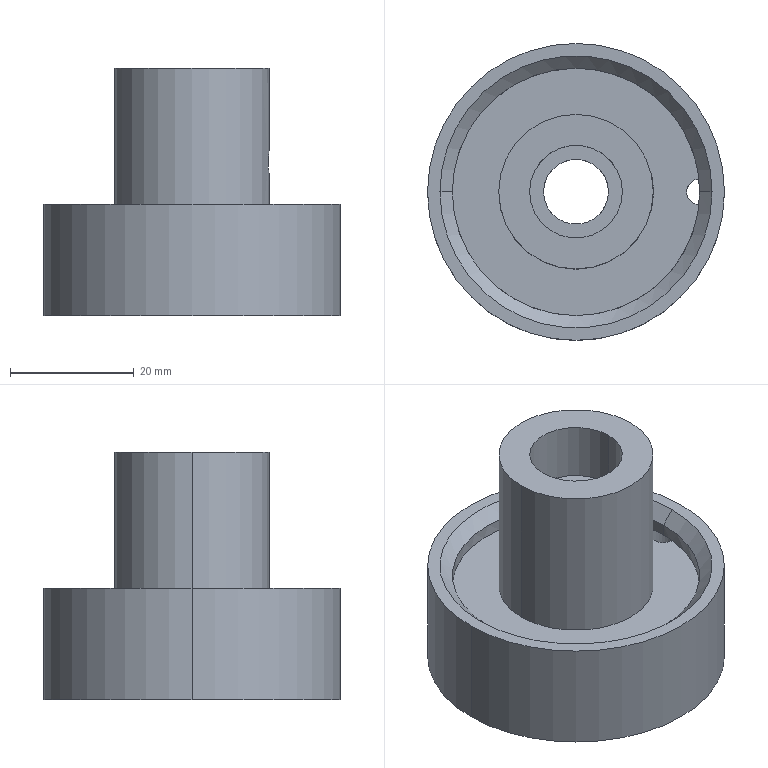Part | 1 solid | 38 faces | box 48 x 48 x 40 mm | volume 34647 mm3 | cylinder 22 | cone 8 | plane 8 | commonest cylinder face diameters 4.2 x8 10.5 x2 12 x2 12.5 x2 15 x2 25 x2
STEP:
#1=CARTESIAN_POINT('',(-6.25,0.,0.));
#2=VERTEX_POINT('',#1);
#3=CARTESIAN_POINT('',(6.25,0.,0.));
#4=VERTEX_POINT('',#3);
#5=CARTESIAN_POINT('',(0.,0.,0.));
#6=DIRECTION('',(0.,0.,1.));
#7=DIRECTION('',(1.,0.,0.));
#8=AXIS2_PLACEMENT_3D('',#5,#6,#7);
#9=CIRCLE('',#8,6.25);
#10=EDGE_CURVE('',#2,#4,#9,.T.);
#11=ORIENTED_EDGE('',*,*,#10,.F.);
#12=CARTESIAN_POINT('',(-6.25,0.,10.5));
#13=VERTEX_POINT('',#12);
#14=CARTESIAN_POINT('',(-6.25,0.,10.5));
#15=DIRECTION('',(0.,0.,1.));
#16=VECTOR('',#15,1000.);
#17=LINE('',#14,#16);
#18=EDGE_CURVE('',#2,#13,#17,.T.);
#19=ORIENTED_EDGE('',*,*,#18,.T.);
#20=CARTESIAN_POINT('',(6.25,0.,10.5));
#21=VERTEX_POINT('',#20);
#22=CARTESIAN_POINT('',(0.,0.,10.5));
#23=DIRECTION('',(0.,0.,1.));
#24=DIRECTION('',(1.,0.,0.));
#25=AXIS2_PLACEMENT_3D('',#22,#23,#24);
#26=CIRCLE('',#25,6.25);
#27=EDGE_CURVE('',#13,#21,#26,.T.);
#28=ORIENTED_EDGE('',*,*,#27,.T.);
#29=CARTESIAN_POINT('',(6.25,0.,10.5));
#30=DIRECTION('',(0.,0.,1.));
#31=VECTOR('',#30,1000.);
#32=LINE('',#29,#31);
#33=EDGE_CURVE('',#4,#21,#32,.T.);
#34=ORIENTED_EDGE('',*,*,#33,.F.);
#35=EDGE_LOOP('',(#11,#19,#28,#34));
#36=FACE_OUTER_BOUND('',#35,.T.);
#37=CARTESIAN_POINT('',(0.,0.,10.5));
#38=DIRECTION('',(0.,0.,1.));
#39=DIRECTION('',(1.,0.,0.));
#40=AXIS2_PLACEMENT_3D('',#37,#38,#39);
#41=CYLINDRICAL_SURFACE('',#40,6.25);
#42=ADVANCED_FACE('',(#36),#41,.F.);
#43=CARTESIAN_POINT('',(6.,0.,10.5));
#44=VERTEX_POINT('',#43);
#45=CARTESIAN_POINT('',(-6.,0.,10.5));
#46=VERTEX_POINT('',#45);
#47=CARTESIAN_POINT('',(0.,0.,10.5));
#48=DIRECTION('',(0.,0.,-1.));
#49=DIRECTION('',(1.,0.,0.));
#50=AXIS2_PLACEMENT_3D('',#47,#48,#49);
#51=CIRCLE('',#50,6.);
#52=EDGE_CURVE('',#44,#46,#51,.T.);
#53=ORIENTED_EDGE('',*,*,#52,.T.);
#54=CARTESIAN_POINT('',(-6.,0.,14.5));
#55=VERTEX_POINT('',#54);
#56=CARTESIAN_POINT('',(-6.,0.,10.5));
#57=DIRECTION('',(0.,0.,1.));
#58=VECTOR('',#57,1000.);
#59=LINE('',#56,#58);
#60=EDGE_CURVE('',#46,#55,#59,.T.);
#61=ORIENTED_EDGE('',*,*,#60,.T.);
#62=CARTESIAN_POINT('',(6.,0.,14.5));
#63=VERTEX_POINT('',#62);
#64=CARTESIAN_POINT('',(0.,0.,14.5));
#65=DIRECTION('',(0.,0.,1.));
#66=DIRECTION('',(1.,0.,0.));
#67=AXIS2_PLACEMENT_3D('',#64,#65,#66);
#68=CIRCLE('',#67,6.);
#69=EDGE_CURVE('',#55,#63,#68,.T.);
#70=ORIENTED_EDGE('',*,*,#69,.T.);
#71=CARTESIAN_POINT('',(6.,0.,10.5));
#72=DIRECTION('',(0.,0.,1.));
#73=VECTOR('',#72,1000.);
#74=LINE('',#71,#73);
#75=EDGE_CURVE('',#44,#63,#74,.T.);
#76=ORIENTED_EDGE('',*,*,#75,.F.);
#77=EDGE_LOOP('',(#53,#61,#70,#76));
#78=FACE_OUTER_BOUND('',#77,.T.);
#79=CARTESIAN_POINT('',(0.,0.,10.5));
#80=DIRECTION('',(0.,0.,1.));
#81=DIRECTION('',(1.,0.,0.));
#82=AXIS2_PLACEMENT_3D('',#79,#80,#81);
#83=CYLINDRICAL_SURFACE('',#82,6.);
#84=ADVANCED_FACE('',(#78),#83,.F.);
#85=CARTESIAN_POINT('',(-5.25,0.,17.5));
#86=VERTEX_POINT('',#85);
#87=CARTESIAN_POINT('',(5.25,0.,17.5));
#88=VERTEX_POINT('',#87);
#89=CARTESIAN_POINT('',(0.,0.,17.5));
#90=DIRECTION('',(0.,0.,1.));
#91=DIRECTION('',(1.,0.,0.));
#92=AXIS2_PLACEMENT_3D('',#89,#90,#91);
#93=CIRCLE('',#92,5.25);
#94=EDGE_CURVE('',#86,#88,#93,.T.);
#95=ORIENTED_EDGE('',*,*,#94,.T.);
#96=CARTESIAN_POINT('',(5.5,0.,14.5));
#97=VERTEX_POINT('',#96);
#98=CARTESIAN_POINT('',(5.5,0.,14.5));
#99=DIRECTION('',(0.08305,0.,-0.9965));
#100=VECTOR('',#99,1000.);
#101=LINE('',#98,#100);
#102=EDGE_CURVE('',#88,#97,#101,.T.);
#103=ORIENTED_EDGE('',*,*,#102,.T.);
#104=CARTESIAN_POINT('',(-5.5,0.,14.5));
#105=VERTEX_POINT('',#104);
#106=CARTESIAN_POINT('',(0.,0.,14.5));
#107=DIRECTION('',(0.,0.,1.));
#108=DIRECTION('',(1.,0.,0.));
#109=AXIS2_PLACEMENT_3D('',#106,#107,#108);
#110=CIRCLE('',#109,5.5);
#111=EDGE_CURVE('',#105,#97,#110,.T.);
#112=ORIENTED_EDGE('',*,*,#111,.F.);
#113=CARTESIAN_POINT('',(-5.5,0.,14.5));
#114=DIRECTION('',(-0.08305,0.,-0.9965));
#115=VECTOR('',#114,1000.);
#116=LINE('',#113,#115);
#117=EDGE_CURVE('',#86,#105,#116,.T.);
#118=ORIENTED_EDGE('',*,*,#117,.F.);
#119=EDGE_LOOP('',(#95,#103,#112,#118));
#120=FACE_OUTER_BOUND('',#119,.T.);
#121=CARTESIAN_POINT('',(0.,0.,14.5));
#122=DIRECTION('',(0.,0.,-1.));
#123=DIRECTION('',(-1.,0.,0.));
#124=AXIS2_PLACEMENT_3D('',#121,#122,#123);
#125=CONICAL_SURFACE('',#124,5.5,0.08314);
#126=ADVANCED_FACE('',(#120),#125,.F.);
#127=CARTESIAN_POINT('',(5.25,0.,22.7));
#128=VERTEX_POINT('',#127);
#129=CARTESIAN_POINT('',(5.25,0.,26.9));
#130=VERTEX_POINT('',#129);
#131=CARTESIAN_POINT('',(5.25,0.,22.7));
#132=CARTESIAN_POINT('',(5.25,-0.1403,22.7));
#133=CARTESIAN_POINT('',(5.244,-0.2781,22.714));
#134=CARTESIAN_POINT('',(5.223,-0.5485,22.768));
#135=CARTESIAN_POINT('',(5.207,-0.6827,22.809));
#136=CARTESIAN_POINT('',(5.167,-0.9365,22.915));
#137=CARTESIAN_POINT('',(5.144,-1.057,22.98));
#138=CARTESIAN_POINT('',(5.092,-1.284,23.133));
#139=CARTESIAN_POINT('',(5.064,-1.39,23.22));
#140=CARTESIAN_POINT('',(4.979,-1.677,23.508));
#141=CARTESIAN_POINT('',(4.921,-1.833,23.739));
#142=CARTESIAN_POINT('',(4.858,-1.991,24.117));
#143=CARTESIAN_POINT('',(4.841,-2.032,24.251));
#144=CARTESIAN_POINT('',(4.818,-2.086,24.523));
#145=CARTESIAN_POINT('',(4.812,-2.1,24.66));
#146=CARTESIAN_POINT('',(4.812,-2.1,24.937));
#147=CARTESIAN_POINT('',(4.818,-2.086,25.078));
#148=CARTESIAN_POINT('',(4.841,-2.032,25.349));
#149=CARTESIAN_POINT('',(4.858,-1.991,25.481));
#150=CARTESIAN_POINT('',(4.9,-1.885,25.736));
#151=CARTESIAN_POINT('',(4.925,-1.82,25.857));
#152=CARTESIAN_POINT('',(4.979,-1.668,26.083));
#153=CARTESIAN_POINT('',(5.007,-1.581,26.189));
#154=CARTESIAN_POINT('',(5.064,-1.388,26.382));
#155=CARTESIAN_POINT('',(5.092,-1.284,26.468));
#156=CARTESIAN_POINT('',(5.144,-1.057,26.62));
#157=CARTESIAN_POINT('',(5.168,-0.9343,26.686));
#158=CARTESIAN_POINT('',(5.227,-0.5556,26.844));
#159=CARTESIAN_POINT('',(5.25,-0.2764,26.9));
#160=CARTESIAN_POINT('',(5.25,0.,26.9));
#161=B_SPLINE_CURVE_WITH_KNOTS('',3,(#131,#132,#133,#134,#135,#136,#137,#138,#139,#140,#141,#142,#143,#144,#145,#146,#147,#148,#149,#150,#151,#152,#153,#154,#155,#156,#157,#158,#159,#160),.UNSPECIFIED.,.F.,.F.,(4,2,2,2,2,2,2,2,2,2,2,2,2,2,4),(0.,0.0004147,0.0008295,0.001244,0.001659,0.002488,0.002903,0.003318,0.003733,0.004147,0.004562,0.004977,0.005392,0.005806,0.006636),.UNSPECIFIED.);
#162=EDGE_CURVE('',#128,#130,#161,.T.);
#163=ORIENTED_EDGE('',*,*,#162,.T.);
#164=CARTESIAN_POINT('',(12.5,0.,26.9));
#165=VERTEX_POINT('',#164);
#166=CARTESIAN_POINT('',(20.,0.,26.9));
#167=DIRECTION('',(1.,0.,0.));
#168=VECTOR('',#167,1000.);
#169=LINE('',#166,#168);
#170=EDGE_CURVE('',#130,#165,#169,.T.);
#171=ORIENTED_EDGE('',*,*,#170,.T.);
#172=CARTESIAN_POINT('',(12.5,0.,22.7));
#173=VERTEX_POINT('',#172);
#174=CARTESIAN_POINT('',(12.5,0.,26.9));
#175=CARTESIAN_POINT('',(12.5,-0.2743,26.9));
#176=CARTESIAN_POINT('',(12.49,-0.5511,26.845));
#177=CARTESIAN_POINT('',(12.466,-0.9302,26.688));
#178=CARTESIAN_POINT('',(12.456,-1.053,26.622));
#179=CARTESIAN_POINT('',(12.435,-1.282,26.469));
#180=CARTESIAN_POINT('',(12.423,-1.387,26.383));
#181=CARTESIAN_POINT('',(12.4,-1.581,26.189));
#182=CARTESIAN_POINT('',(12.388,-1.669,26.081));
#183=CARTESIAN_POINT('',(12.367,-1.822,25.854));
#184=CARTESIAN_POINT('',(12.357,-1.886,25.733));
#185=CARTESIAN_POINT('',(12.34,-1.992,25.479));
#186=CARTESIAN_POINT('',(12.334,-2.032,25.346));
#187=CARTESIAN_POINT('',(12.325,-2.086,25.077));
#188=CARTESIAN_POINT('',(12.322,-2.1,24.94));
#189=CARTESIAN_POINT('',(12.322,-2.1,24.663));
#190=CARTESIAN_POINT('',(12.325,-2.087,24.526));
#191=CARTESIAN_POINT('',(12.334,-2.033,24.257));
#192=CARTESIAN_POINT('',(12.34,-1.993,24.123));
#193=CARTESIAN_POINT('',(12.357,-1.888,23.869));
#194=CARTESIAN_POINT('',(12.367,-1.823,23.749));
#195=CARTESIAN_POINT('',(12.388,-1.671,23.52));
#196=CARTESIAN_POINT('',(12.4,-1.582,23.413));
#197=CARTESIAN_POINT('',(12.434,-1.293,23.123));
#198=CARTESIAN_POINT('',(12.458,-1.059,22.966));
#199=CARTESIAN_POINT('',(12.482,-0.6803,22.809));
#200=CARTESIAN_POINT('',(12.489,-0.5475,22.768));
#201=CARTESIAN_POINT('',(12.498,-0.2763,22.714));
#202=CARTESIAN_POINT('',(12.5,-0.139,22.7));
#203=CARTESIAN_POINT('',(12.5,0.,22.7));
#204=B_SPLINE_CURVE_WITH_KNOTS('',3,(#174,#175,#176,#177,#178,#179,#180,#181,#182,#183,#184,#185,#186,#187,#188,#189,#190,#191,#192,#193,#194,#195,#196,#197,#198,#199,#200,#201,#202,#203),.UNSPECIFIED.,.F.,.F.,(4,2,2,2,2,2,2,2,2,2,2,2,2,2,4),(0.006577,0.007399,0.00781,0.008221,0.008632,0.009043,0.009454,0.009865,0.01028,0.01069,0.0111,0.01151,0.01233,0.01274,0.01315),.UNSPECIFIED.);
#205=EDGE_CURVE('',#165,#173,#204,.T.);
#206=ORIENTED_EDGE('',*,*,#205,.T.);
#207=CARTESIAN_POINT('',(20.,0.,22.7));
#208=DIRECTION('',(1.,0.,0.));
#209=VECTOR('',#208,1000.);
#210=LINE('',#207,#209);
#211=EDGE_CURVE('',#128,#173,#210,.T.);
#212=ORIENTED_EDGE('',*,*,#211,.F.);
#213=EDGE_LOOP('',(#163,#171,#206,#212));
#214=FACE_OUTER_BOUND('',#213,.T.);
#215=CARTESIAN_POINT('',(20.,0.,24.8));
#216=DIRECTION('',(1.,0.,0.));
#217=DIRECTION('',(0.,0.,-1.));
#218=AXIS2_PLACEMENT_3D('',#215,#216,#217);
#219=CYLINDRICAL_SURFACE('',#218,2.1);
#220=ADVANCED_FACE('',(#214),#219,.F.);
#221=CARTESIAN_POINT('',(-7.5,0.,30.5));
#222=VERTEX_POINT('',#221);
#223=CARTESIAN_POINT('',(7.5,0.,30.5));
#224=VERTEX_POINT('',#223);
#225=CARTESIAN_POINT('',(0.,0.,30.5));
#226=DIRECTION('',(0.,0.,1.));
#227=DIRECTION('',(1.,0.,0.));
#228=AXIS2_PLACEMENT_3D('',#225,#226,#227);
#229=CIRCLE('',#228,7.5);
#230=EDGE_CURVE('',#222,#224,#229,.T.);
#231=ORIENTED_EDGE('',*,*,#230,.F.);
#232=CARTESIAN_POINT('',(-7.5,0.,40.));
#233=VERTEX_POINT('',#232);
#234=CARTESIAN_POINT('',(-7.5,0.,30.5));
#235=DIRECTION('',(0.,0.,1.));
#236=VECTOR('',#235,1000.);
#237=LINE('',#234,#236);
#238=EDGE_CURVE('',#222,#233,#237,.T.);
#239=ORIENTED_EDGE('',*,*,#238,.T.);
#240=CARTESIAN_POINT('',(7.5,0.,40.));
#241=VERTEX_POINT('',#240);
#242=CARTESIAN_POINT('',(0.,0.,40.));
#243=DIRECTION('',(0.,0.,1.));
#244=DIRECTION('',(1.,0.,0.));
#245=AXIS2_PLACEMENT_3D('',#242,#243,#244);
#246=CIRCLE('',#245,7.5);
#247=EDGE_CURVE('',#233,#241,#246,.T.);
#248=ORIENTED_EDGE('',*,*,#247,.T.);
#249=CARTESIAN_POINT('',(7.5,0.,30.5));
#250=DIRECTION('',(0.,0.,1.));
#251=VECTOR('',#250,1000.);
#252=LINE('',#249,#251);
#253=EDGE_CURVE('',#224,#241,#252,.T.);
#254=ORIENTED_EDGE('',*,*,#253,.F.);
#255=EDGE_LOOP('',(#231,#239,#248,#254));
#256=FACE_OUTER_BOUND('',#255,.T.);
#257=CARTESIAN_POINT('',(0.,0.,30.5));
#258=DIRECTION('',(0.,0.,1.));
#259=DIRECTION('',(1.,0.,0.));
#260=AXIS2_PLACEMENT_3D('',#257,#258,#259);
#261=CYLINDRICAL_SURFACE('',#260,7.5);
#262=ADVANCED_FACE('',(#256),#261,.F.);
#263=CARTESIAN_POINT('',(-20.,0.,16.));
#264=VERTEX_POINT('',#263);
#265=CARTESIAN_POINT('',(20.,0.,16.));
#266=VERTEX_POINT('',#265);
#267=CARTESIAN_POINT('',(0.,0.,16.));
#268=DIRECTION('',(0.,0.,1.));
#269=DIRECTION('',(1.,0.,0.));
#270=AXIS2_PLACEMENT_3D('',#267,#268,#269);
#271=CIRCLE('',#270,20.);
#272=EDGE_CURVE('',#264,#266,#271,.T.);
#273=ORIENTED_EDGE('',*,*,#272,.F.);
#274=CARTESIAN_POINT('',(-22.,0.,18.));
#275=VERTEX_POINT('',#274);
#276=CARTESIAN_POINT('',(-20.,0.,16.));
#277=DIRECTION('',(-0.7071,0.,0.7071));
#278=VECTOR('',#277,1000.);
#279=LINE('',#276,#278);
#280=EDGE_CURVE('',#264,#275,#279,.T.);
#281=ORIENTED_EDGE('',*,*,#280,.T.);
#282=CARTESIAN_POINT('',(22.,0.,18.));
#283=VERTEX_POINT('',#282);
#284=CARTESIAN_POINT('',(0.,0.,18.));
#285=DIRECTION('',(0.,0.,-1.));
#286=DIRECTION('',(1.,0.,0.));
#287=AXIS2_PLACEMENT_3D('',#284,#285,#286);
#288=CIRCLE('',#287,22.);
#289=EDGE_CURVE('',#283,#275,#288,.T.);
#290=ORIENTED_EDGE('',*,*,#289,.F.);
#291=CARTESIAN_POINT('',(20.,0.,16.));
#292=DIRECTION('',(0.7071,0.,0.7071));
#293=VECTOR('',#292,1000.);
#294=LINE('',#291,#293);
#295=EDGE_CURVE('',#266,#283,#294,.T.);
#296=ORIENTED_EDGE('',*,*,#295,.F.);
#297=EDGE_LOOP('',(#273,#281,#290,#296));
#298=FACE_OUTER_BOUND('',#297,.T.);
#299=CARTESIAN_POINT('',(0.,0.,16.));
#300=DIRECTION('',(0.,0.,1.));
#301=DIRECTION('',(1.,0.,0.));
#302=AXIS2_PLACEMENT_3D('',#299,#300,#301);
#303=CONICAL_SURFACE('',#302,20.,0.7854);
#304=ADVANCED_FACE('',(#298),#303,.F.);
#305=CARTESIAN_POINT('',(17.9,0.,0.));
#306=VERTEX_POINT('',#305);
#307=CARTESIAN_POINT('',(22.1,0.,0.));
#308=VERTEX_POINT('',#307);
#309=CARTESIAN_POINT('',(20.,0.,0.));
#310=DIRECTION('',(0.,0.,1.));
#311=DIRECTION('',(1.,0.,0.));
#312=AXIS2_PLACEMENT_3D('',#309,#310,#311);
#313=CIRCLE('',#312,2.1);
#314=EDGE_CURVE('',#306,#308,#313,.T.);
#315=ORIENTED_EDGE('',*,*,#314,.F.);
#316=CARTESIAN_POINT('',(17.9,0.,14.));
#317=VERTEX_POINT('',#316);
#318=CARTESIAN_POINT('',(17.9,0.,14.));
#319=DIRECTION('',(0.,0.,1.));
#320=VECTOR('',#319,1000.);
#321=LINE('',#318,#320);
#322=EDGE_CURVE('',#306,#317,#321,.T.);
#323=ORIENTED_EDGE('',*,*,#322,.T.);
#324=CARTESIAN_POINT('',(19.89,-2.097,14.));
#325=VERTEX_POINT('',#324);
#326=CARTESIAN_POINT('',(20.,0.,14.));
#327=DIRECTION('',(0.,0.,1.));
#328=DIRECTION('',(1.,0.,0.));
#329=AXIS2_PLACEMENT_3D('',#326,#327,#328);
#330=CIRCLE('',#329,2.1);
#331=EDGE_CURVE('',#317,#325,#330,.T.);
#332=ORIENTED_EDGE('',*,*,#331,.T.);
#333=CARTESIAN_POINT('',(22.1,0.,14.));
#334=VERTEX_POINT('',#333);
#335=CARTESIAN_POINT('',(20.,0.,14.));
#336=DIRECTION('',(0.,0.,1.));
#337=DIRECTION('',(1.,0.,0.));
#338=AXIS2_PLACEMENT_3D('',#335,#336,#337);
#339=CIRCLE('',#338,2.1);
#340=EDGE_CURVE('',#325,#334,#339,.T.);
#341=ORIENTED_EDGE('',*,*,#340,.T.);
#342=CARTESIAN_POINT('',(22.1,0.,14.));
#343=DIRECTION('',(0.,0.,1.));
#344=VECTOR('',#343,1000.);
#345=LINE('',#342,#344);
#346=EDGE_CURVE('',#308,#334,#345,.T.);
#347=ORIENTED_EDGE('',*,*,#346,.F.);
#348=EDGE_LOOP('',(#315,#323,#332,#341,#347));
#349=FACE_OUTER_BOUND('',#348,.T.);
#350=CARTESIAN_POINT('',(20.,0.,14.));
#351=DIRECTION('',(0.,0.,1.));
#352=DIRECTION('',(1.,0.,0.));
#353=AXIS2_PLACEMENT_3D('',#350,#351,#352);
#354=CYLINDRICAL_SURFACE('',#353,2.1);
#355=ADVANCED_FACE('',(#349),#354,.F.);
#356=CARTESIAN_POINT('',(2.717,19.99,10.));
#357=VERTEX_POINT('',#356);
#358=CARTESIAN_POINT('',(-1.483,19.99,10.));
#359=VERTEX_POINT('',#358);
#360=CARTESIAN_POINT('',(0.6172,19.99,10.));
#361=DIRECTION('',(0.,0.,-1.));
#362=DIRECTION('',(-1.,0.,0.));
#363=AXIS2_PLACEMENT_3D('',#360,#361,#362);
#364=CIRCLE('',#363,2.1);
#365=EDGE_CURVE('',#357,#359,#364,.T.);
#366=ORIENTED_EDGE('',*,*,#365,.F.);
#367=CARTESIAN_POINT('',(2.717,19.99,0.));
#368=VERTEX_POINT('',#367);
#369=CARTESIAN_POINT('',(2.717,19.99,0.));
#370=DIRECTION('',(0.,0.,-1.));
#371=VECTOR('',#370,1000.);
#372=LINE('',#369,#371);
#373=EDGE_CURVE('',#357,#368,#372,.T.);
#374=ORIENTED_EDGE('',*,*,#373,.T.);
#375=CARTESIAN_POINT('',(-1.483,19.99,0.));
#376=VERTEX_POINT('',#375);
#377=CARTESIAN_POINT('',(0.6172,19.99,0.));
#378=DIRECTION('',(0.,0.,-1.));
#379=DIRECTION('',(-1.,0.,0.));
#380=AXIS2_PLACEMENT_3D('',#377,#378,#379);
#381=CIRCLE('',#380,2.1);
#382=EDGE_CURVE('',#368,#376,#381,.T.);
#383=ORIENTED_EDGE('',*,*,#382,.T.);
#384=CARTESIAN_POINT('',(-1.483,19.99,0.));
#385=DIRECTION('',(0.,0.,-1.));
#386=VECTOR('',#385,1000.);
#387=LINE('',#384,#386);
#388=EDGE_CURVE('',#359,#376,#387,.T.);
#389=ORIENTED_EDGE('',*,*,#388,.F.);
#390=EDGE_LOOP('',(#366,#374,#383,#389));
#391=FACE_OUTER_BOUND('',#390,.T.);
#392=CARTESIAN_POINT('',(0.6172,19.99,0.));
#393=DIRECTION('',(0.,0.,-1.));
#394=DIRECTION('',(-1.,0.,0.));
#395=AXIS2_PLACEMENT_3D('',#392,#393,#394);
#396=CYLINDRICAL_SURFACE('',#395,2.1);
#397=ADVANCED_FACE('',(#391),#396,.F.);
#398=CARTESIAN_POINT('',(0.6172,19.99,11.262));
#399=VERTEX_POINT('',#398);
#400=CARTESIAN_POINT('',(-1.483,19.99,10.));
#401=DIRECTION('',(-0.8572,0.,-0.515));
#402=VECTOR('',#401,1000.);
#403=LINE('',#400,#402);
#404=EDGE_CURVE('',#399,#359,#403,.T.);
#405=ORIENTED_EDGE('',*,*,#404,.F.);
#406=CARTESIAN_POINT('',(2.717,19.99,10.));
#407=DIRECTION('',(0.8572,0.,-0.515));
#408=VECTOR('',#407,1000.);
#409=LINE('',#406,#408);
#410=EDGE_CURVE('',#399,#357,#409,.T.);
#411=ORIENTED_EDGE('',*,*,#410,.T.);
#412=ORIENTED_EDGE('',*,*,#365,.T.);
#413=EDGE_LOOP('',(#405,#411,#412));
#414=FACE_OUTER_BOUND('',#413,.T.);
#415=CARTESIAN_POINT('',(0.6172,19.99,10.));
#416=DIRECTION('',(0.,0.,-1.));
#417=DIRECTION('',(-1.,0.,0.));
#418=AXIS2_PLACEMENT_3D('',#415,#416,#417);
#419=CONICAL_SURFACE('',#418,2.1,1.03);
#420=ADVANCED_FACE('',(#414),#419,.F.);
#421=CARTESIAN_POINT('',(2.72,-20.028,10.));
#422=VERTEX_POINT('',#421);
#423=CARTESIAN_POINT('',(-1.48,-20.028,10.));
#424=VERTEX_POINT('',#423);
#425=CARTESIAN_POINT('',(0.6196,-20.028,10.));
#426=DIRECTION('',(0.,0.,-1.));
#427=DIRECTION('',(-1.,0.,0.));
#428=AXIS2_PLACEMENT_3D('',#425,#426,#427);
#429=CIRCLE('',#428,2.1);
#430=EDGE_CURVE('',#422,#424,#429,.T.);
#431=ORIENTED_EDGE('',*,*,#430,.F.);
#432=CARTESIAN_POINT('',(2.72,-20.028,0.));
#433=VERTEX_POINT('',#432);
#434=CARTESIAN_POINT('',(2.72,-20.028,0.));
#435=DIRECTION('',(0.,0.,-1.));
#436=VECTOR('',#435,1000.);
#437=LINE('',#434,#436);
#438=EDGE_CURVE('',#422,#433,#437,.T.);
#439=ORIENTED_EDGE('',*,*,#438,.T.);
#440=CARTESIAN_POINT('',(-1.48,-20.028,0.));
#441=VERTEX_POINT('',#440);
#442=CARTESIAN_POINT('',(0.6196,-20.028,0.));
#443=DIRECTION('',(0.,0.,-1.));
#444=DIRECTION('',(-1.,0.,0.));
#445=AXIS2_PLACEMENT_3D('',#442,#443,#444);
#446=CIRCLE('',#445,2.1);
#447=EDGE_CURVE('',#433,#441,#446,.T.);
#448=ORIENTED_EDGE('',*,*,#447,.T.);
#449=CARTESIAN_POINT('',(-1.48,-20.028,0.));
#450=DIRECTION('',(0.,0.,-1.));
#451=VECTOR('',#450,1000.);
#452=LINE('',#449,#451);
#453=EDGE_CURVE('',#424,#441,#452,.T.);
#454=ORIENTED_EDGE('',*,*,#453,.F.);
#455=EDGE_LOOP('',(#431,#439,#448,#454));
#456=FACE_OUTER_BOUND('',#455,.T.);
#457=CARTESIAN_POINT('',(0.6196,-20.028,0.));
#458=DIRECTION('',(0.,0.,-1.));
#459=DIRECTION('',(-1.,0.,0.));
#460=AXIS2_PLACEMENT_3D('',#457,#458,#459);
#461=CYLINDRICAL_SURFACE('',#460,2.1);
#462=ADVANCED_FACE('',(#456),#461,.F.);
#463=CARTESIAN_POINT('',(0.6196,-20.028,11.262));
#464=VERTEX_POINT('',#463);
#465=CARTESIAN_POINT('',(-1.48,-20.028,10.));
#466=DIRECTION('',(-0.8572,0.,-0.515));
#467=VECTOR('',#466,1000.);
#468=LINE('',#465,#467);
#469=EDGE_CURVE('',#464,#424,#468,.T.);
#470=ORIENTED_EDGE('',*,*,#469,.F.);
#471=CARTESIAN_POINT('',(2.72,-20.028,10.));
#472=DIRECTION('',(0.8572,0.,-0.515));
#473=VECTOR('',#472,1000.);
#474=LINE('',#471,#473);
#475=EDGE_CURVE('',#464,#422,#474,.T.);
#476=ORIENTED_EDGE('',*,*,#475,.T.);
#477=ORIENTED_EDGE('',*,*,#430,.T.);
#478=EDGE_LOOP('',(#470,#476,#477));
#479=FACE_OUTER_BOUND('',#478,.T.);
#480=CARTESIAN_POINT('',(0.6196,-20.028,10.));
#481=DIRECTION('',(0.,0.,-1.));
#482=DIRECTION('',(-1.,0.,0.));
#483=AXIS2_PLACEMENT_3D('',#480,#481,#482);
#484=CONICAL_SURFACE('',#483,2.1,1.03);
#485=ADVANCED_FACE('',(#479),#484,.F.);
#486=CARTESIAN_POINT('',(24.,0.,18.));
#487=VERTEX_POINT('',#486);
#488=CARTESIAN_POINT('',(-24.,0.,18.));
#489=VERTEX_POINT('',#488);
#490=CARTESIAN_POINT('',(0.,0.,18.));
#491=DIRECTION('',(0.,0.,1.));
#492=DIRECTION('',(1.,0.,0.));
#493=AXIS2_PLACEMENT_3D('',#490,#491,#492);
#494=CIRCLE('',#493,24.);
#495=EDGE_CURVE('',#487,#489,#494,.T.);
#496=ORIENTED_EDGE('',*,*,#495,.F.);
#497=CARTESIAN_POINT('',(24.,0.,0.));
#498=VERTEX_POINT('',#497);
#499=CARTESIAN_POINT('',(24.,0.,40.));
#500=DIRECTION('',(0.,0.,-1.));
#501=VECTOR('',#500,1000.);
#502=LINE('',#499,#501);
#503=EDGE_CURVE('',#487,#498,#502,.T.);
#504=ORIENTED_EDGE('',*,*,#503,.T.);
#505=CARTESIAN_POINT('',(-24.,0.,0.));
#506=VERTEX_POINT('',#505);
#507=CARTESIAN_POINT('',(0.,0.,0.));
#508=DIRECTION('',(0.,0.,1.));
#509=DIRECTION('',(1.,0.,0.));
#510=AXIS2_PLACEMENT_3D('',#507,#508,#509);
#511=CIRCLE('',#510,24.);
#512=EDGE_CURVE('',#498,#506,#511,.T.);
#513=ORIENTED_EDGE('',*,*,#512,.T.);
#514=CARTESIAN_POINT('',(-24.,0.,40.));
#515=DIRECTION('',(0.,0.,-1.));
#516=VECTOR('',#515,1000.);
#517=LINE('',#514,#516);
#518=EDGE_CURVE('',#489,#506,#517,.T.);
#519=ORIENTED_EDGE('',*,*,#518,.F.);
#520=EDGE_LOOP('',(#496,#504,#513,#519));
#521=FACE_OUTER_BOUND('',#520,.T.);
#522=CARTESIAN_POINT('',(0.,0.,40.));
#523=DIRECTION('',(0.,0.,-1.));
#524=DIRECTION('',(-1.,0.,0.));
#525=AXIS2_PLACEMENT_3D('',#522,#523,#524);
#526=CYLINDRICAL_SURFACE('',#525,24.);
#527=ADVANCED_FACE('',(#521),#526,.T.);
#528=CARTESIAN_POINT('',(-12.5,0.,14.));
#529=VERTEX_POINT('',#528);
#530=CARTESIAN_POINT('',(12.5,0.,14.));
#531=VERTEX_POINT('',#530);
#532=CARTESIAN_POINT('',(0.,0.,14.));
#533=DIRECTION('',(0.,0.,-1.));
#534=DIRECTION('',(1.,0.,0.));
#535=AXIS2_PLACEMENT_3D('',#532,#533,#534);
#536=CIRCLE('',#535,12.5);
#537=EDGE_CURVE('',#529,#531,#536,.T.);
#538=ORIENTED_EDGE('',*,*,#537,.F.);
#539=CARTESIAN_POINT('',(-12.5,0.,40.));
#540=VERTEX_POINT('',#539);
#541=CARTESIAN_POINT('',(-12.5,0.,-56.569));
#542=DIRECTION('',(0.,0.,1.));
#543=VECTOR('',#542,1000.);
#544=LINE('',#541,#543);
#545=EDGE_CURVE('',#529,#540,#544,.T.);
#546=ORIENTED_EDGE('',*,*,#545,.T.);
#547=CARTESIAN_POINT('',(12.5,0.,40.));
#548=VERTEX_POINT('',#547);
#549=CARTESIAN_POINT('',(0.,0.,40.));
#550=DIRECTION('',(0.,0.,1.));
#551=DIRECTION('',(1.,0.,0.));
#552=AXIS2_PLACEMENT_3D('',#549,#550,#551);
#553=CIRCLE('',#552,12.5);
#554=EDGE_CURVE('',#548,#540,#553,.T.);
#555=ORIENTED_EDGE('',*,*,#554,.F.);
#556=CARTESIAN_POINT('',(12.5,0.,-56.569));
#557=DIRECTION('',(0.,0.,1.));
#558=VECTOR('',#557,1000.);
#559=LINE('',#556,#558);
#560=EDGE_CURVE('',#165,#548,#559,.T.);
#561=ORIENTED_EDGE('',*,*,#560,.F.);
#562=CARTESIAN_POINT('',(12.5,0.,22.7));
#563=CARTESIAN_POINT('',(12.5,0.139,22.7));
#564=CARTESIAN_POINT('',(12.498,0.2757,22.714));
#565=CARTESIAN_POINT('',(12.489,0.5444,22.767));
#566=CARTESIAN_POINT('',(12.482,0.6779,22.808));
#567=CARTESIAN_POINT('',(12.466,0.9322,22.913));
#568=CARTESIAN_POINT('',(12.456,1.053,22.978));
#569=CARTESIAN_POINT('',(12.435,1.281,23.13));
#570=CARTESIAN_POINT('',(12.423,1.389,23.219));
#571=CARTESIAN_POINT('',(12.388,1.679,23.509));
#572=CARTESIAN_POINT('',(12.365,1.835,23.743));
#573=CARTESIAN_POINT('',(12.332,2.045,24.248));
#574=CARTESIAN_POINT('',(12.322,2.1,24.525));
#575=CARTESIAN_POINT('',(12.322,2.1,24.936));
#576=CARTESIAN_POINT('',(12.325,2.086,25.076));
#577=CARTESIAN_POINT('',(12.334,2.033,25.345));
#578=CARTESIAN_POINT('',(12.34,1.993,25.476));
#579=CARTESIAN_POINT('',(12.357,1.887,25.731));
#580=CARTESIAN_POINT('',(12.367,1.822,25.854));
#581=CARTESIAN_POINT('',(12.388,1.67,26.081));
#582=CARTESIAN_POINT('',(12.4,1.583,26.187));
#583=CARTESIAN_POINT('',(12.423,1.387,26.383));
#584=CARTESIAN_POINT('',(12.435,1.281,26.469));
#585=CARTESIAN_POINT('',(12.456,1.054,26.621));
#586=CARTESIAN_POINT('',(12.466,0.9312,26.687));
#587=CARTESIAN_POINT('',(12.482,0.6771,26.793));
#588=CARTESIAN_POINT('',(12.489,0.5462,26.832));
#589=CARTESIAN_POINT('',(12.498,0.2765,26.886));
#590=CARTESIAN_POINT('',(12.5,0.1372,26.9));
#591=CARTESIAN_POINT('',(12.5,0.,26.9));
#592=B_SPLINE_CURVE_WITH_KNOTS('',3,(#562,#563,#564,#565,#566,#567,#568,#569,#570,#571,#572,#573,#574,#575,#576,#577,#578,#579,#580,#581,#582,#583,#584,#585,#586,#587,#588,#589,#590,#591),.UNSPECIFIED.,.F.,.F.,(4,2,2,2,2,2,2,2,2,2,2,2,2,2,4),(0.,0.0004111,0.0008222,0.001233,0.001644,0.002466,0.003289,0.0037,0.004111,0.004522,0.004933,0.005344,0.005755,0.006166,0.006577),.UNSPECIFIED.);
#593=EDGE_CURVE('',#173,#165,#592,.T.);
#594=ORIENTED_EDGE('',*,*,#593,.F.);
#595=CARTESIAN_POINT('',(12.5,0.,-56.569));
#596=DIRECTION('',(0.,0.,1.));
#597=VECTOR('',#596,1000.);
#598=LINE('',#595,#597);
#599=EDGE_CURVE('',#531,#173,#598,.T.);
#600=ORIENTED_EDGE('',*,*,#599,.F.);
#601=EDGE_LOOP('',(#538,#546,#555,#561,#594,#600));
#602=FACE_OUTER_BOUND('',#601,.T.);
#603=CARTESIAN_POINT('',(0.,0.,-56.569));
#604=DIRECTION('',(0.,0.,1.));
#605=DIRECTION('',(1.,0.,0.));
#606=AXIS2_PLACEMENT_3D('',#603,#604,#605);
#607=CYLINDRICAL_SURFACE('',#606,12.5);
#608=ADVANCED_FACE('',(#602),#607,.T.);
#609=CARTESIAN_POINT('',(-20.,0.,14.));
#610=VERTEX_POINT('',#609);
#611=CARTESIAN_POINT('',(0.,0.,14.));
#612=DIRECTION('',(0.,0.,-1.));
#613=DIRECTION('',(1.,0.,0.));
#614=AXIS2_PLACEMENT_3D('',#611,#612,#613);
#615=CIRCLE('',#614,20.);
#616=EDGE_CURVE('',#325,#610,#615,.T.);
#617=ORIENTED_EDGE('',*,*,#616,.T.);
#618=CARTESIAN_POINT('',(-20.,0.,-56.569));
#619=DIRECTION('',(0.,0.,1.));
#620=VECTOR('',#619,1000.);
#621=LINE('',#618,#620);
#622=EDGE_CURVE('',#610,#264,#621,.T.);
#623=ORIENTED_EDGE('',*,*,#622,.T.);
#624=ORIENTED_EDGE('',*,*,#272,.T.);
#625=CARTESIAN_POINT('',(20.,0.,14.));
#626=VERTEX_POINT('',#625);
#627=CARTESIAN_POINT('',(20.,0.,-56.569));
#628=DIRECTION('',(0.,0.,1.));
#629=VECTOR('',#628,1000.);
#630=LINE('',#627,#629);
#631=EDGE_CURVE('',#626,#266,#630,.T.);
#632=ORIENTED_EDGE('',*,*,#631,.F.);
#633=CARTESIAN_POINT('',(0.,0.,14.));
#634=DIRECTION('',(0.,0.,-1.));
#635=DIRECTION('',(1.,0.,0.));
#636=AXIS2_PLACEMENT_3D('',#633,#634,#635);
#637=CIRCLE('',#636,20.);
#638=EDGE_CURVE('',#626,#325,#637,.T.);
#639=ORIENTED_EDGE('',*,*,#638,.T.);
#640=EDGE_LOOP('',(#617,#623,#624,#632,#639));
#641=FACE_OUTER_BOUND('',#640,.T.);
#642=CARTESIAN_POINT('',(0.,0.,-56.569));
#643=DIRECTION('',(0.,0.,1.));
#644=DIRECTION('',(1.,0.,0.));
#645=AXIS2_PLACEMENT_3D('',#642,#643,#644);
#646=CYLINDRICAL_SURFACE('',#645,20.);
#647=ADVANCED_FACE('',(#641),#646,.F.);
#648=ORIENTED_EDGE('',*,*,#94,.F.);
#649=CARTESIAN_POINT('',(-5.25,0.,30.5));
#650=VERTEX_POINT('',#649);
#651=CARTESIAN_POINT('',(-5.25,0.,14.5));
#652=DIRECTION('',(0.,0.,1.));
#653=VECTOR('',#652,1000.);
#654=LINE('',#651,#653);
#655=EDGE_CURVE('',#86,#650,#654,.T.);
#656=ORIENTED_EDGE('',*,*,#655,.T.);
#657=CARTESIAN_POINT('',(5.25,0.,30.5));
#658=VERTEX_POINT('',#657);
#659=CARTESIAN_POINT('',(0.,0.,30.5));
#660=DIRECTION('',(0.,0.,1.));
#661=DIRECTION('',(1.,0.,0.));
#662=AXIS2_PLACEMENT_3D('',#659,#660,#661);
#663=CIRCLE('',#662,5.25);
#664=EDGE_CURVE('',#650,#658,#663,.T.);
#665=ORIENTED_EDGE('',*,*,#664,.T.);
#666=CARTESIAN_POINT('',(5.25,0.,14.5));
#667=DIRECTION('',(0.,0.,1.));
#668=VECTOR('',#667,1000.);
#669=LINE('',#666,#668);
#670=EDGE_CURVE('',#130,#658,#669,.T.);
#671=ORIENTED_EDGE('',*,*,#670,.F.);
#672=ORIENTED_EDGE('',*,*,#162,.F.);
#673=CARTESIAN_POINT('',(5.25,0.,14.5));
#674=DIRECTION('',(0.,0.,1.));
#675=VECTOR('',#674,1000.);
#676=LINE('',#673,#675);
#677=EDGE_CURVE('',#88,#128,#676,.T.);
#678=ORIENTED_EDGE('',*,*,#677,.F.);
#679=EDGE_LOOP('',(#648,#656,#665,#671,#672,#678));
#680=FACE_OUTER_BOUND('',#679,.T.);
#681=CARTESIAN_POINT('',(0.,0.,14.5));
#682=DIRECTION('',(0.,0.,1.));
#683=DIRECTION('',(1.,0.,0.));
#684=AXIS2_PLACEMENT_3D('',#681,#682,#683);
#685=CYLINDRICAL_SURFACE('',#684,5.25);
#686=ADVANCED_FACE('',(#680),#685,.F.);
#687=ORIENTED_EDGE('',*,*,#655,.F.);
#688=CARTESIAN_POINT('',(0.,0.,17.5));
#689=DIRECTION('',(0.,0.,1.));
#690=DIRECTION('',(1.,0.,0.));
#691=AXIS2_PLACEMENT_3D('',#688,#689,#690);
#692=CIRCLE('',#691,5.25);
#693=EDGE_CURVE('',#88,#86,#692,.T.);
#694=ORIENTED_EDGE('',*,*,#693,.F.);
#695=ORIENTED_EDGE('',*,*,#677,.T.);
#696=CARTESIAN_POINT('',(5.25,0.,26.9));
#697=CARTESIAN_POINT('',(5.25,0.1381,26.9));
#698=CARTESIAN_POINT('',(5.244,0.2782,26.886));
#699=CARTESIAN_POINT('',(5.223,0.5503,26.831));
#700=CARTESIAN_POINT('',(5.207,0.6817,26.791));
#701=CARTESIAN_POINT('',(5.168,0.9358,26.685));
#702=CARTESIAN_POINT('',(5.144,1.058,26.619));
#703=CARTESIAN_POINT('',(5.092,1.284,26.467));
#704=CARTESIAN_POINT('',(5.064,1.389,26.381));
#705=CARTESIAN_POINT('',(5.007,1.583,26.187));
#706=CARTESIAN_POINT('',(4.978,1.669,26.082));
#707=CARTESIAN_POINT('',(4.925,1.82,25.857));
#708=CARTESIAN_POINT('',(4.9,1.886,25.734));
#709=CARTESIAN_POINT('',(4.858,1.991,25.481));
#710=CARTESIAN_POINT('',(4.841,2.031,25.35));
#711=CARTESIAN_POINT('',(4.818,2.086,25.079));
#712=CARTESIAN_POINT('',(4.812,2.1,24.939));
#713=CARTESIAN_POINT('',(4.812,2.1,24.523));
#714=CARTESIAN_POINT('',(4.837,2.044,24.245));
#715=CARTESIAN_POINT('',(4.9,1.886,23.866));
#716=CARTESIAN_POINT('',(4.925,1.82,23.743));
#717=CARTESIAN_POINT('',(4.979,1.668,23.517));
#718=CARTESIAN_POINT('',(5.007,1.582,23.412));
#719=CARTESIAN_POINT('',(5.064,1.389,23.219));
#720=CARTESIAN_POINT('',(5.092,1.283,23.132));
#721=CARTESIAN_POINT('',(5.144,1.057,22.98));
#722=CARTESIAN_POINT('',(5.167,0.9372,22.916));
#723=CARTESIAN_POINT('',(5.227,0.5536,22.755));
#724=CARTESIAN_POINT('',(5.25,0.2805,22.7));
#725=CARTESIAN_POINT('',(5.25,0.,22.7));
#726=B_SPLINE_CURVE_WITH_KNOTS('',3,(#696,#697,#698,#699,#700,#701,#702,#703,#704,#705,#706,#707,#708,#709,#710,#711,#712,#713,#714,#715,#716,#717,#718,#719,#720,#721,#722,#723,#724,#725),.UNSPECIFIED.,.F.,.F.,(4,2,2,2,2,2,2,2,2,2,2,2,2,2,4),(0.006636,0.00705,0.007465,0.007879,0.008294,0.008708,0.009123,0.009537,0.009951,0.01078,0.01119,0.01161,0.01202,0.01244,0.01327),.UNSPECIFIED.);
#727=EDGE_CURVE('',#130,#128,#726,.T.);
#728=ORIENTED_EDGE('',*,*,#727,.F.);
#729=ORIENTED_EDGE('',*,*,#670,.T.);
#730=CARTESIAN_POINT('',(0.,0.,30.5));
#731=DIRECTION('',(0.,0.,1.));
#732=DIRECTION('',(1.,0.,0.));
#733=AXIS2_PLACEMENT_3D('',#730,#731,#732);
#734=CIRCLE('',#733,5.25);
#735=EDGE_CURVE('',#658,#650,#734,.T.);
#736=ORIENTED_EDGE('',*,*,#735,.T.);
#737=EDGE_LOOP('',(#687,#694,#695,#728,#729,#736));
#738=FACE_OUTER_BOUND('',#737,.T.);
#739=CARTESIAN_POINT('',(0.,0.,14.5));
#740=DIRECTION('',(0.,0.,1.));
#741=DIRECTION('',(1.,0.,0.));
#742=AXIS2_PLACEMENT_3D('',#739,#740,#741);
#743=CYLINDRICAL_SURFACE('',#742,5.25);
#744=ADVANCED_FACE('',(#738),#743,.F.);
#745=ORIENTED_EDGE('',*,*,#622,.F.);
#746=CARTESIAN_POINT('',(19.89,2.097,14.));
#747=VERTEX_POINT('',#746);
#748=CARTESIAN_POINT('',(0.,0.,14.));
#749=DIRECTION('',(0.,0.,-1.));
#750=DIRECTION('',(1.,0.,0.));
#751=AXIS2_PLACEMENT_3D('',#748,#749,#750);
#752=CIRCLE('',#751,20.);
#753=EDGE_CURVE('',#610,#747,#752,.T.);
#754=ORIENTED_EDGE('',*,*,#753,.T.);
#755=CARTESIAN_POINT('',(0.,0.,14.));
#756=DIRECTION('',(0.,0.,-1.));
#757=DIRECTION('',(1.,0.,0.));
#758=AXIS2_PLACEMENT_3D('',#755,#756,#757);
#759=CIRCLE('',#758,20.);
#760=EDGE_CURVE('',#747,#626,#759,.T.);
#761=ORIENTED_EDGE('',*,*,#760,.T.);
#762=ORIENTED_EDGE('',*,*,#631,.T.);
#763=CARTESIAN_POINT('',(0.,0.,16.));
#764=DIRECTION('',(0.,0.,1.));
#765=DIRECTION('',(1.,0.,0.));
#766=AXIS2_PLACEMENT_3D('',#763,#764,#765);
#767=CIRCLE('',#766,20.);
#768=EDGE_CURVE('',#266,#264,#767,.T.);
#769=ORIENTED_EDGE('',*,*,#768,.T.);
#770=EDGE_LOOP('',(#745,#754,#761,#762,#769));
#771=FACE_OUTER_BOUND('',#770,.T.);
#772=CARTESIAN_POINT('',(0.,0.,-56.569));
#773=DIRECTION('',(0.,0.,1.));
#774=DIRECTION('',(1.,0.,0.));
#775=AXIS2_PLACEMENT_3D('',#772,#773,#774);
#776=CYLINDRICAL_SURFACE('',#775,20.);
#777=ADVANCED_FACE('',(#771),#776,.F.);
#778=ORIENTED_EDGE('',*,*,#545,.F.);
#779=CARTESIAN_POINT('',(0.,0.,14.));
#780=DIRECTION('',(0.,0.,-1.));
#781=DIRECTION('',(1.,0.,0.));
#782=AXIS2_PLACEMENT_3D('',#779,#780,#781);
#783=CIRCLE('',#782,12.5);
#784=EDGE_CURVE('',#531,#529,#783,.T.);
#785=ORIENTED_EDGE('',*,*,#784,.F.);
#786=ORIENTED_EDGE('',*,*,#599,.T.);
#787=ORIENTED_EDGE('',*,*,#205,.F.);
#788=ORIENTED_EDGE('',*,*,#560,.T.);
#789=CARTESIAN_POINT('',(0.,0.,40.));
#790=DIRECTION('',(0.,0.,1.));
#791=DIRECTION('',(1.,0.,0.));
#792=AXIS2_PLACEMENT_3D('',#789,#790,#791);
#793=CIRCLE('',#792,12.5);
#794=EDGE_CURVE('',#540,#548,#793,.T.);
#795=ORIENTED_EDGE('',*,*,#794,.F.);
#796=EDGE_LOOP('',(#778,#785,#786,#787,#788,#795));
#797=FACE_OUTER_BOUND('',#796,.T.);
#798=CARTESIAN_POINT('',(0.,0.,-56.569));
#799=DIRECTION('',(0.,0.,1.));
#800=DIRECTION('',(1.,0.,0.));
#801=AXIS2_PLACEMENT_3D('',#798,#799,#800);
#802=CYLINDRICAL_SURFACE('',#801,12.5);
#803=ADVANCED_FACE('',(#797),#802,.T.);
#804=CARTESIAN_POINT('',(20.,0.,14.));
#805=DIRECTION('',(0.,0.,1.));
#806=DIRECTION('',(1.,0.,0.));
#807=AXIS2_PLACEMENT_3D('',#804,#805,#806);
#808=CIRCLE('',#807,2.1);
#809=EDGE_CURVE('',#747,#317,#808,.T.);
#810=ORIENTED_EDGE('',*,*,#809,.F.);
#811=ORIENTED_EDGE('',*,*,#753,.F.);
#812=ORIENTED_EDGE('',*,*,#616,.F.);
#813=ORIENTED_EDGE('',*,*,#331,.F.);
#814=EDGE_LOOP('',(#810,#811,#812,#813));
#815=FACE_OUTER_BOUND('',#814,.T.);
#816=ORIENTED_EDGE('',*,*,#784,.T.);
#817=ORIENTED_EDGE('',*,*,#537,.T.);
#818=EDGE_LOOP('',(#816,#817));
#819=FACE_BOUND('',#818,.T.);
#820=CARTESIAN_POINT('',(0.,0.,14.));
#821=DIRECTION('',(0.,0.,1.));
#822=DIRECTION('',(1.,0.,0.));
#823=AXIS2_PLACEMENT_3D('',#820,#821,#822);
#824=PLANE('',#823);
#825=ADVANCED_FACE('',(#815,#819),#824,.T.);
#826=CARTESIAN_POINT('',(0.,0.,40.));
#827=DIRECTION('',(0.,0.,1.));
#828=DIRECTION('',(1.,0.,0.));
#829=AXIS2_PLACEMENT_3D('',#826,#827,#828);
#830=CIRCLE('',#829,7.5);
#831=EDGE_CURVE('',#241,#233,#830,.T.);
#832=ORIENTED_EDGE('',*,*,#831,.F.);
#833=ORIENTED_EDGE('',*,*,#247,.F.);
#834=EDGE_LOOP('',(#832,#833));
#835=FACE_BOUND('',#834,.T.);
#836=ORIENTED_EDGE('',*,*,#554,.T.);
#837=ORIENTED_EDGE('',*,*,#794,.T.);
#838=EDGE_LOOP('',(#836,#837));
#839=FACE_OUTER_BOUND('',#838,.T.);
#840=CARTESIAN_POINT('',(0.,0.,40.));
#841=DIRECTION('',(0.,0.,1.));
#842=DIRECTION('',(1.,0.,0.));
#843=AXIS2_PLACEMENT_3D('',#840,#841,#842);
#844=PLANE('',#843);
#845=ADVANCED_FACE('',(#835,#839),#844,.T.);
#846=ORIENTED_EDGE('',*,*,#289,.T.);
#847=CARTESIAN_POINT('',(0.,0.,18.));
#848=DIRECTION('',(0.,0.,-1.));
#849=DIRECTION('',(1.,0.,0.));
#850=AXIS2_PLACEMENT_3D('',#847,#848,#849);
#851=CIRCLE('',#850,22.);
#852=EDGE_CURVE('',#275,#283,#851,.T.);
#853=ORIENTED_EDGE('',*,*,#852,.T.);
#854=EDGE_LOOP('',(#846,#853));
#855=FACE_BOUND('',#854,.T.);
#856=CARTESIAN_POINT('',(0.,0.,18.));
#857=DIRECTION('',(0.,0.,1.));
#858=DIRECTION('',(1.,0.,0.));
#859=AXIS2_PLACEMENT_3D('',#856,#857,#858);
#860=CIRCLE('',#859,24.);
#861=EDGE_CURVE('',#489,#487,#860,.T.);
#862=ORIENTED_EDGE('',*,*,#861,.T.);
#863=ORIENTED_EDGE('',*,*,#495,.T.);
#864=EDGE_LOOP('',(#862,#863));
#865=FACE_OUTER_BOUND('',#864,.T.);
#866=CARTESIAN_POINT('',(0.,0.,18.));
#867=DIRECTION('',(0.,0.,1.));
#868=DIRECTION('',(1.,0.,0.));
#869=AXIS2_PLACEMENT_3D('',#866,#867,#868);
#870=PLANE('',#869);
#871=ADVANCED_FACE('',(#855,#865),#870,.T.);
#872=CARTESIAN_POINT('',(0.,0.,0.));
#873=DIRECTION('',(0.,0.,1.));
#874=DIRECTION('',(1.,0.,0.));
#875=AXIS2_PLACEMENT_3D('',#872,#873,#874);
#876=CIRCLE('',#875,6.25);
#877=EDGE_CURVE('',#4,#2,#876,.T.);
#878=ORIENTED_EDGE('',*,*,#877,.T.);
#879=ORIENTED_EDGE('',*,*,#10,.T.);
#880=EDGE_LOOP('',(#878,#879));
#881=FACE_BOUND('',#880,.T.);
#882=CARTESIAN_POINT('',(20.,0.,0.));
#883=DIRECTION('',(0.,0.,1.));
#884=DIRECTION('',(1.,0.,0.));
#885=AXIS2_PLACEMENT_3D('',#882,#883,#884);
#886=CIRCLE('',#885,2.1);
#887=EDGE_CURVE('',#308,#306,#886,.T.);
#888=ORIENTED_EDGE('',*,*,#887,.T.);
#889=ORIENTED_EDGE('',*,*,#314,.T.);
#890=EDGE_LOOP('',(#888,#889));
#891=FACE_BOUND('',#890,.T.);
#892=CARTESIAN_POINT('',(0.6172,19.99,0.));
#893=DIRECTION('',(0.,0.,-1.));
#894=DIRECTION('',(-1.,0.,0.));
#895=AXIS2_PLACEMENT_3D('',#892,#893,#894);
#896=CIRCLE('',#895,2.1);
#897=EDGE_CURVE('',#376,#368,#896,.T.);
#898=ORIENTED_EDGE('',*,*,#897,.F.);
#899=ORIENTED_EDGE('',*,*,#382,.F.);
#900=EDGE_LOOP('',(#898,#899));
#901=FACE_BOUND('',#900,.T.);
#902=CARTESIAN_POINT('',(0.6196,-20.028,0.));
#903=DIRECTION('',(0.,0.,-1.));
#904=DIRECTION('',(-1.,0.,0.));
#905=AXIS2_PLACEMENT_3D('',#902,#903,#904);
#906=CIRCLE('',#905,2.1);
#907=EDGE_CURVE('',#441,#433,#906,.T.);
#908=ORIENTED_EDGE('',*,*,#907,.F.);
#909=ORIENTED_EDGE('',*,*,#447,.F.);
#910=EDGE_LOOP('',(#908,#909));
#911=FACE_BOUND('',#910,.T.);
#912=CARTESIAN_POINT('',(0.,0.,0.));
#913=DIRECTION('',(0.,0.,1.));
#914=DIRECTION('',(1.,0.,0.));
#915=AXIS2_PLACEMENT_3D('',#912,#913,#914);
#916=CIRCLE('',#915,24.);
#917=EDGE_CURVE('',#506,#498,#916,.T.);
#918=ORIENTED_EDGE('',*,*,#917,.F.);
#919=ORIENTED_EDGE('',*,*,#512,.F.);
#920=EDGE_LOOP('',(#918,#919));
#921=FACE_OUTER_BOUND('',#920,.T.);
#922=CARTESIAN_POINT('',(0.,0.,0.));
#923=DIRECTION('',(0.,0.,1.));
#924=DIRECTION('',(1.,0.,0.));
#925=AXIS2_PLACEMENT_3D('',#922,#923,#924);
#926=PLANE('',#925);
#927=ADVANCED_FACE('',(#881,#891,#901,#911,#921),#926,.F.);
#928=ORIENTED_EDGE('',*,*,#503,.F.);
#929=ORIENTED_EDGE('',*,*,#861,.F.);
#930=ORIENTED_EDGE('',*,*,#518,.T.);
#931=ORIENTED_EDGE('',*,*,#917,.T.);
#932=EDGE_LOOP('',(#928,#929,#930,#931));
#933=FACE_OUTER_BOUND('',#932,.T.);
#934=CARTESIAN_POINT('',(0.,0.,40.));
#935=DIRECTION('',(0.,0.,-1.));
#936=DIRECTION('',(-1.,0.,0.));
#937=AXIS2_PLACEMENT_3D('',#934,#935,#936);
#938=CYLINDRICAL_SURFACE('',#937,24.);
#939=ADVANCED_FACE('',(#933),#938,.T.);
#940=ORIENTED_EDGE('',*,*,#475,.F.);
#941=ORIENTED_EDGE('',*,*,#469,.T.);
#942=CARTESIAN_POINT('',(0.6196,-20.028,10.));
#943=DIRECTION('',(0.,0.,-1.));
#944=DIRECTION('',(-1.,0.,0.));
#945=AXIS2_PLACEMENT_3D('',#942,#943,#944);
#946=CIRCLE('',#945,2.1);
#947=EDGE_CURVE('',#424,#422,#946,.T.);
#948=ORIENTED_EDGE('',*,*,#947,.T.);
#949=EDGE_LOOP('',(#940,#941,#948));
#950=FACE_OUTER_BOUND('',#949,.T.);
#951=CARTESIAN_POINT('',(0.6196,-20.028,10.));
#952=DIRECTION('',(0.,0.,-1.));
#953=DIRECTION('',(-1.,0.,0.));
#954=AXIS2_PLACEMENT_3D('',#951,#952,#953);
#955=CONICAL_SURFACE('',#954,2.1,1.03);
#956=ADVANCED_FACE('',(#950),#955,.F.);
#957=ORIENTED_EDGE('',*,*,#438,.F.);
#958=ORIENTED_EDGE('',*,*,#947,.F.);
#959=ORIENTED_EDGE('',*,*,#453,.T.);
#960=ORIENTED_EDGE('',*,*,#907,.T.);
#961=EDGE_LOOP('',(#957,#958,#959,#960));
#962=FACE_OUTER_BOUND('',#961,.T.);
#963=CARTESIAN_POINT('',(0.6196,-20.028,0.));
#964=DIRECTION('',(0.,0.,-1.));
#965=DIRECTION('',(-1.,0.,0.));
#966=AXIS2_PLACEMENT_3D('',#963,#964,#965);
#967=CYLINDRICAL_SURFACE('',#966,2.1);
#968=ADVANCED_FACE('',(#962),#967,.F.);
#969=ORIENTED_EDGE('',*,*,#410,.F.);
#970=ORIENTED_EDGE('',*,*,#404,.T.);
#971=CARTESIAN_POINT('',(0.6172,19.99,10.));
#972=DIRECTION('',(0.,0.,-1.));
#973=DIRECTION('',(-1.,0.,0.));
#974=AXIS2_PLACEMENT_3D('',#971,#972,#973);
#975=CIRCLE('',#974,2.1);
#976=EDGE_CURVE('',#359,#357,#975,.T.);
#977=ORIENTED_EDGE('',*,*,#976,.T.);
#978=EDGE_LOOP('',(#969,#970,#977));
#979=FACE_OUTER_BOUND('',#978,.T.);
#980=CARTESIAN_POINT('',(0.6172,19.99,10.));
#981=DIRECTION('',(0.,0.,-1.));
#982=DIRECTION('',(-1.,0.,0.));
#983=AXIS2_PLACEMENT_3D('',#980,#981,#982);
#984=CONICAL_SURFACE('',#983,2.1,1.03);
#985=ADVANCED_FACE('',(#979),#984,.F.);
#986=ORIENTED_EDGE('',*,*,#373,.F.);
#987=ORIENTED_EDGE('',*,*,#976,.F.);
#988=ORIENTED_EDGE('',*,*,#388,.T.);
#989=ORIENTED_EDGE('',*,*,#897,.T.);
#990=EDGE_LOOP('',(#986,#987,#988,#989));
#991=FACE_OUTER_BOUND('',#990,.T.);
#992=CARTESIAN_POINT('',(0.6172,19.99,0.));
#993=DIRECTION('',(0.,0.,-1.));
#994=DIRECTION('',(-1.,0.,0.));
#995=AXIS2_PLACEMENT_3D('',#992,#993,#994);
#996=CYLINDRICAL_SURFACE('',#995,2.1);
#997=ADVANCED_FACE('',(#991),#996,.F.);
#998=ORIENTED_EDGE('',*,*,#340,.F.);
#999=ORIENTED_EDGE('',*,*,#638,.F.);
#1000=ORIENTED_EDGE('',*,*,#760,.F.);
#1001=CARTESIAN_POINT('',(20.,0.,14.));
#1002=DIRECTION('',(0.,0.,1.));
#1003=DIRECTION('',(1.,0.,0.));
#1004=AXIS2_PLACEMENT_3D('',#1001,#1002,#1003);
#1005=CIRCLE('',#1004,2.1);
#1006=EDGE_CURVE('',#334,#747,#1005,.T.);
#1007=ORIENTED_EDGE('',*,*,#1006,.F.);
#1008=EDGE_LOOP('',(#998,#999,#1000,#1007));
#1009=FACE_OUTER_BOUND('',#1008,.T.);
#1010=CARTESIAN_POINT('',(22.1,0.,14.));
#1011=DIRECTION('',(0.,0.,1.));
#1012=DIRECTION('',(1.,0.,0.));
#1013=AXIS2_PLACEMENT_3D('',#1010,#1011,#1012);
#1014=PLANE('',#1013);
#1015=ADVANCED_FACE('',(#1009),#1014,.F.);
#1016=ORIENTED_EDGE('',*,*,#322,.F.);
#1017=ORIENTED_EDGE('',*,*,#887,.F.);
#1018=ORIENTED_EDGE('',*,*,#346,.T.);
#1019=ORIENTED_EDGE('',*,*,#1006,.T.);
#1020=ORIENTED_EDGE('',*,*,#809,.T.);
#1021=EDGE_LOOP('',(#1016,#1017,#1018,#1019,#1020));
#1022=FACE_OUTER_BOUND('',#1021,.T.);
#1023=CARTESIAN_POINT('',(20.,0.,14.));
#1024=DIRECTION('',(0.,0.,1.));
#1025=DIRECTION('',(1.,0.,0.));
#1026=AXIS2_PLACEMENT_3D('',#1023,#1024,#1025);
#1027=CYLINDRICAL_SURFACE('',#1026,2.1);
#1028=ADVANCED_FACE('',(#1022),#1027,.F.);
#1029=ORIENTED_EDGE('',*,*,#280,.F.);
#1030=ORIENTED_EDGE('',*,*,#768,.F.);
#1031=ORIENTED_EDGE('',*,*,#295,.T.);
#1032=ORIENTED_EDGE('',*,*,#852,.F.);
#1033=EDGE_LOOP('',(#1029,#1030,#1031,#1032));
#1034=FACE_OUTER_BOUND('',#1033,.T.);
#1035=CARTESIAN_POINT('',(0.,0.,16.));
#1036=DIRECTION('',(0.,0.,1.));
#1037=DIRECTION('',(1.,0.,0.));
#1038=AXIS2_PLACEMENT_3D('',#1035,#1036,#1037);
#1039=CONICAL_SURFACE('',#1038,20.,0.7854);
#1040=ADVANCED_FACE('',(#1034),#1039,.F.);
#1041=ORIENTED_EDGE('',*,*,#238,.F.);
#1042=CARTESIAN_POINT('',(0.,0.,30.5));
#1043=DIRECTION('',(0.,0.,1.));
#1044=DIRECTION('',(1.,0.,0.));
#1045=AXIS2_PLACEMENT_3D('',#1042,#1043,#1044);
#1046=CIRCLE('',#1045,7.5);
#1047=EDGE_CURVE('',#224,#222,#1046,.T.);
#1048=ORIENTED_EDGE('',*,*,#1047,.F.);
#1049=ORIENTED_EDGE('',*,*,#253,.T.);
#1050=ORIENTED_EDGE('',*,*,#831,.T.);
#1051=EDGE_LOOP('',(#1041,#1048,#1049,#1050));
#1052=FACE_OUTER_BOUND('',#1051,.T.);
#1053=CARTESIAN_POINT('',(0.,0.,30.5));
#1054=DIRECTION('',(0.,0.,1.));
#1055=DIRECTION('',(1.,0.,0.));
#1056=AXIS2_PLACEMENT_3D('',#1053,#1054,#1055);
#1057=CYLINDRICAL_SURFACE('',#1056,7.5);
#1058=ADVANCED_FACE('',(#1052),#1057,.F.);
#1059=ORIENTED_EDGE('',*,*,#735,.F.);
#1060=ORIENTED_EDGE('',*,*,#664,.F.);
#1061=EDGE_LOOP('',(#1059,#1060));
#1062=FACE_BOUND('',#1061,.T.);
#1063=ORIENTED_EDGE('',*,*,#1047,.T.);
#1064=ORIENTED_EDGE('',*,*,#230,.T.);
#1065=EDGE_LOOP('',(#1063,#1064));
#1066=FACE_OUTER_BOUND('',#1065,.T.);
#1067=CARTESIAN_POINT('',(0.,0.,30.5));
#1068=DIRECTION('',(0.,0.,1.));
#1069=DIRECTION('',(1.,0.,0.));
#1070=AXIS2_PLACEMENT_3D('',#1067,#1068,#1069);
#1071=PLANE('',#1070);
#1072=ADVANCED_FACE('',(#1062,#1066),#1071,.T.);
#1073=ORIENTED_EDGE('',*,*,#170,.F.);
#1074=ORIENTED_EDGE('',*,*,#727,.T.);
#1075=ORIENTED_EDGE('',*,*,#211,.T.);
#1076=ORIENTED_EDGE('',*,*,#593,.T.);
#1077=EDGE_LOOP('',(#1073,#1074,#1075,#1076));
#1078=FACE_OUTER_BOUND('',#1077,.T.);
#1079=CARTESIAN_POINT('',(20.,0.,24.8));
#1080=DIRECTION('',(1.,0.,0.));
#1081=DIRECTION('',(0.,0.,-1.));
#1082=AXIS2_PLACEMENT_3D('',#1079,#1080,#1081);
#1083=CYLINDRICAL_SURFACE('',#1082,2.1);
#1084=ADVANCED_FACE('',(#1078),#1083,.F.);
#1085=ORIENTED_EDGE('',*,*,#102,.F.);
#1086=ORIENTED_EDGE('',*,*,#693,.T.);
#1087=ORIENTED_EDGE('',*,*,#117,.T.);
#1088=CARTESIAN_POINT('',(0.,0.,14.5));
#1089=DIRECTION('',(0.,0.,1.));
#1090=DIRECTION('',(1.,0.,0.));
#1091=AXIS2_PLACEMENT_3D('',#1088,#1089,#1090);
#1092=CIRCLE('',#1091,5.5);
#1093=EDGE_CURVE('',#97,#105,#1092,.T.);
#1094=ORIENTED_EDGE('',*,*,#1093,.F.);
#1095=EDGE_LOOP('',(#1085,#1086,#1087,#1094));
#1096=FACE_OUTER_BOUND('',#1095,.T.);
#1097=CARTESIAN_POINT('',(0.,0.,14.5));
#1098=DIRECTION('',(0.,0.,-1.));
#1099=DIRECTION('',(-1.,0.,0.));
#1100=AXIS2_PLACEMENT_3D('',#1097,#1098,#1099);
#1101=CONICAL_SURFACE('',#1100,5.5,0.08314);
#1102=ADVANCED_FACE('',(#1096),#1101,.F.);
#1103=ORIENTED_EDGE('',*,*,#60,.F.);
#1104=CARTESIAN_POINT('',(0.,0.,10.5));
#1105=DIRECTION('',(0.,0.,-1.));
#1106=DIRECTION('',(1.,0.,0.));
#1107=AXIS2_PLACEMENT_3D('',#1104,#1105,#1106);
#1108=CIRCLE('',#1107,6.);
#1109=EDGE_CURVE('',#46,#44,#1108,.T.);
#1110=ORIENTED_EDGE('',*,*,#1109,.T.);
#1111=ORIENTED_EDGE('',*,*,#75,.T.);
#1112=CARTESIAN_POINT('',(0.,0.,14.5));
#1113=DIRECTION('',(0.,0.,1.));
#1114=DIRECTION('',(1.,0.,0.));
#1115=AXIS2_PLACEMENT_3D('',#1112,#1113,#1114);
#1116=CIRCLE('',#1115,6.);
#1117=EDGE_CURVE('',#63,#55,#1116,.T.);
#1118=ORIENTED_EDGE('',*,*,#1117,.T.);
#1119=EDGE_LOOP('',(#1103,#1110,#1111,#1118));
#1120=FACE_OUTER_BOUND('',#1119,.T.);
#1121=CARTESIAN_POINT('',(0.,0.,10.5));
#1122=DIRECTION('',(0.,0.,1.));
#1123=DIRECTION('',(1.,0.,0.));
#1124=AXIS2_PLACEMENT_3D('',#1121,#1122,#1123);
#1125=CYLINDRICAL_SURFACE('',#1124,6.);
#1126=ADVANCED_FACE('',(#1120),#1125,.F.);
#1127=ORIENTED_EDGE('',*,*,#111,.T.);
#1128=ORIENTED_EDGE('',*,*,#1093,.T.);
#1129=EDGE_LOOP('',(#1127,#1128));
#1130=FACE_BOUND('',#1129,.T.);
#1131=ORIENTED_EDGE('',*,*,#1117,.F.);
#1132=ORIENTED_EDGE('',*,*,#69,.F.);
#1133=EDGE_LOOP('',(#1131,#1132));
#1134=FACE_OUTER_BOUND('',#1133,.T.);
#1135=CARTESIAN_POINT('',(0.,0.,14.5));
#1136=DIRECTION('',(0.,0.,1.));
#1137=DIRECTION('',(1.,0.,0.));
#1138=AXIS2_PLACEMENT_3D('',#1135,#1136,#1137);
#1139=PLANE('',#1138);
#1140=ADVANCED_FACE('',(#1130,#1134),#1139,.F.);
#1141=CARTESIAN_POINT('',(0.,0.,10.5));
#1142=DIRECTION('',(0.,0.,1.));
#1143=DIRECTION('',(1.,0.,0.));
#1144=AXIS2_PLACEMENT_3D('',#1141,#1142,#1143);
#1145=CIRCLE('',#1144,6.25);
#1146=EDGE_CURVE('',#21,#13,#1145,.T.);
#1147=ORIENTED_EDGE('',*,*,#1146,.F.);
#1148=ORIENTED_EDGE('',*,*,#27,.F.);
#1149=EDGE_LOOP('',(#1147,#1148));
#1150=FACE_OUTER_BOUND('',#1149,.T.);
#1151=ORIENTED_EDGE('',*,*,#52,.F.);
#1152=ORIENTED_EDGE('',*,*,#1109,.F.);
#1153=EDGE_LOOP('',(#1151,#1152));
#1154=FACE_BOUND('',#1153,.T.);
#1155=CARTESIAN_POINT('',(6.25,0.,10.5));
#1156=DIRECTION('',(0.,0.,1.));
#1157=DIRECTION('',(1.,0.,0.));
#1158=AXIS2_PLACEMENT_3D('',#1155,#1156,#1157);
#1159=PLANE('',#1158);
#1160=ADVANCED_FACE('',(#1150,#1154),#1159,.F.);
#1161=ORIENTED_EDGE('',*,*,#18,.F.);
#1162=ORIENTED_EDGE('',*,*,#877,.F.);
#1163=ORIENTED_EDGE('',*,*,#33,.T.);
#1164=ORIENTED_EDGE('',*,*,#1146,.T.);
#1165=EDGE_LOOP('',(#1161,#1162,#1163,#1164));
#1166=FACE_OUTER_BOUND('',#1165,.T.);
#1167=CARTESIAN_POINT('',(0.,0.,10.5));
#1168=DIRECTION('',(0.,0.,1.));
#1169=DIRECTION('',(1.,0.,0.));
#1170=AXIS2_PLACEMENT_3D('',#1167,#1168,#1169);
#1171=CYLINDRICAL_SURFACE('',#1170,6.25);
#1172=ADVANCED_FACE('',(#1166),#1171,.F.);
#1173=CLOSED_SHELL('',(#42,#84,#126,#220,#262,#304,#355,#397,#420,#462,#485,#527,#608,#647,#686,#744,#777,#803,#825,#845,#871,#927,#939,#956,#968,#985,#997,#1015,#1028,#1040,#1058,#1072,#1084,#1102,#1126,#1140,#1160,#1172));
#1174=MANIFOLD_SOLID_BREP('',#1173);
#1175=CARTESIAN_POINT('',(0.,0.,0.));
#1176=DIRECTION('',(0.,0.,1.));
#1177=DIRECTION('',(1.,0.,0.));
#1178=AXIS2_PLACEMENT_3D('',#1175,#1176,#1177);
#1179=(LENGTH_UNIT()NAMED_UNIT(*)SI_UNIT(.MILLI.,.METRE.));
#1180=UNCERTAINTY_MEASURE_WITH_UNIT(LENGTH_MEASURE(0.00001),#1179,'','');
#1181=(NAMED_UNIT(*)PLANE_ANGLE_UNIT()SI_UNIT($,.RADIAN.));
#1182=(NAMED_UNIT(*)SI_UNIT($,.STERADIAN.)SOLID_ANGLE_UNIT());
#1183=(GEOMETRIC_REPRESENTATION_CONTEXT(3)GLOBAL_UNCERTAINTY_ASSIGNED_CONTEXT((#1180))GLOBAL_UNIT_ASSIGNED_CONTEXT((#1179,#1181,#1182))REPRESENTATION_CONTEXT('',''));
#1184=ADVANCED_BREP_SHAPE_REPRESENTATION('',(#1174,#1178),#1183);